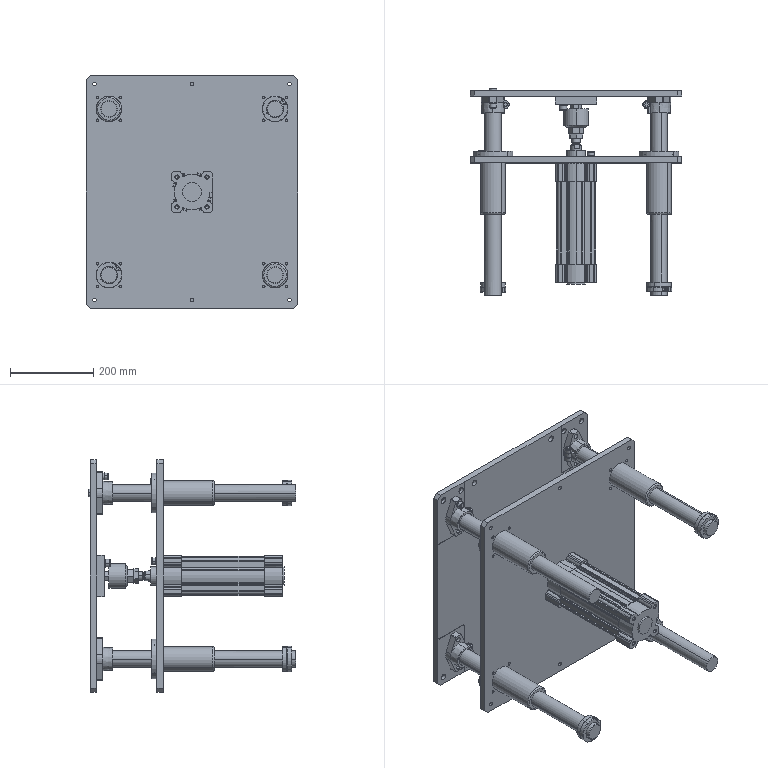Part | SolidWorks | 31 solids | 1391 faces | box 510 x 499.1 x 560 mm | volume 13976626 mm3 | cylinder 646 | plane 520 | cone 175 | torus 38 | spline 12 | commonest cylinder face diameters 9 x72 14 x40 10 x38 40 x38 18 x34 6.8 x32